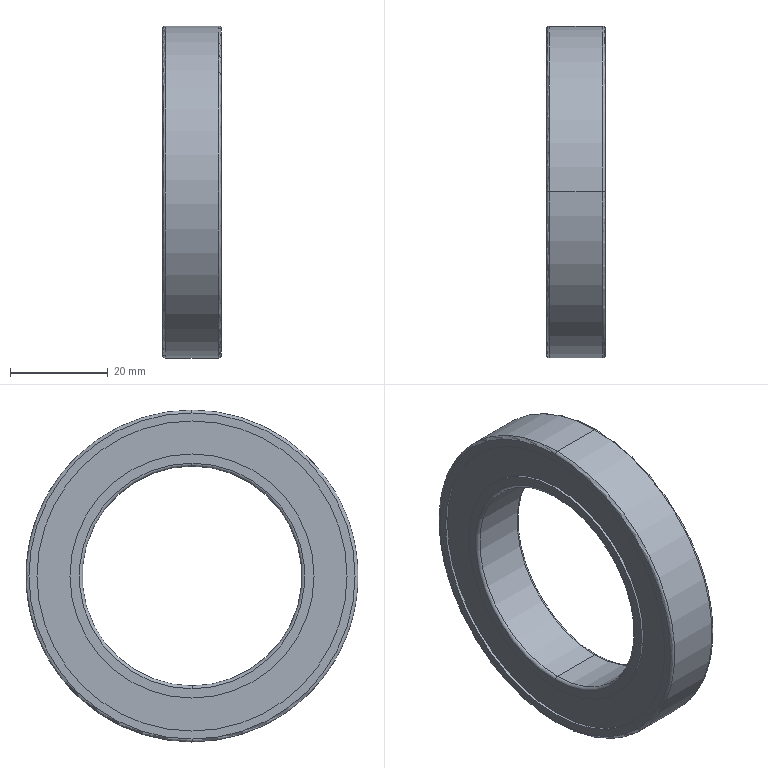Part | SolidWorks | features Fillet 2, Revolution 1 | 1 solid | 26 faces | box 12 x 68 x 68 mm | volume 23116 mm3 | cylinder 12 | torus 8 | plane 6 | commonest cylinder face diameters 50 x4 63.5 x4 45 x2 68 x2
STEP:
#1=CARTESIAN_POINT('',(0.6,0.,22.5));
#2=VERTEX_POINT('',#1);
#3=CARTESIAN_POINT('',(0.6,0.,-22.5));
#4=VERTEX_POINT('',#3);
#5=CARTESIAN_POINT('',(0.6,0.,0.));
#6=DIRECTION('',(-1.,0.,0.));
#7=DIRECTION('',(0.,0.,-1.));
#8=AXIS2_PLACEMENT_3D('',#5,#6,#7);
#9=CIRCLE('',#8,22.5);
#10=EDGE_CURVE('',#2,#4,#9,.T.);
#11=ORIENTED_EDGE('',*,*,#10,.F.);
#12=CARTESIAN_POINT('',(0.,0.,23.1));
#13=VERTEX_POINT('',#12);
#14=CARTESIAN_POINT('',(0.6,0.,23.1));
#15=DIRECTION('',(0.,1.,0.));
#16=DIRECTION('',(0.,0.,1.));
#17=AXIS2_PLACEMENT_3D('',#14,#15,#16);
#18=CIRCLE('',#17,0.6);
#19=EDGE_CURVE('',#2,#13,#18,.T.);
#20=ORIENTED_EDGE('',*,*,#19,.T.);
#21=CARTESIAN_POINT('',(0.,0.,-23.1));
#22=VERTEX_POINT('',#21);
#23=CARTESIAN_POINT('',(0.,0.,0.));
#24=DIRECTION('',(1.,0.,0.));
#25=DIRECTION('',(0.,0.,-1.));
#26=AXIS2_PLACEMENT_3D('',#23,#24,#25);
#27=CIRCLE('',#26,23.1);
#28=EDGE_CURVE('',#22,#13,#27,.T.);
#29=ORIENTED_EDGE('',*,*,#28,.F.);
#30=CARTESIAN_POINT('',(0.6,0.,-23.1));
#31=DIRECTION('',(0.,-1.,0.));
#32=DIRECTION('',(0.,0.,-1.));
#33=AXIS2_PLACEMENT_3D('',#30,#31,#32);
#34=CIRCLE('',#33,0.6);
#35=EDGE_CURVE('',#4,#22,#34,.T.);
#36=ORIENTED_EDGE('',*,*,#35,.F.);
#37=EDGE_LOOP('',(#11,#20,#29,#36));
#38=FACE_OUTER_BOUND('',#37,.T.);
#39=CARTESIAN_POINT('',(0.6,0.,0.));
#40=DIRECTION('',(1.,0.,0.));
#41=DIRECTION('',(0.,0.,-1.));
#42=AXIS2_PLACEMENT_3D('',#39,#40,#41);
#43=TOROIDAL_SURFACE('',#42,23.1,0.6);
#44=ADVANCED_FACE('',(#38),#43,.T.);
#45=CARTESIAN_POINT('',(11.4,0.,-22.5));
#46=VERTEX_POINT('',#45);
#47=CARTESIAN_POINT('',(11.4,0.,22.5));
#48=VERTEX_POINT('',#47);
#49=CARTESIAN_POINT('',(11.4,0.,0.));
#50=DIRECTION('',(1.,0.,0.));
#51=DIRECTION('',(0.,0.,1.));
#52=AXIS2_PLACEMENT_3D('',#49,#50,#51);
#53=CIRCLE('',#52,22.5);
#54=EDGE_CURVE('',#46,#48,#53,.T.);
#55=ORIENTED_EDGE('',*,*,#54,.F.);
#56=CARTESIAN_POINT('',(12.,0.,-23.1));
#57=VERTEX_POINT('',#56);
#58=CARTESIAN_POINT('',(11.4,0.,-23.1));
#59=DIRECTION('',(0.,1.,0.));
#60=DIRECTION('',(0.,0.,1.));
#61=AXIS2_PLACEMENT_3D('',#58,#59,#60);
#62=CIRCLE('',#61,0.6);
#63=EDGE_CURVE('',#46,#57,#62,.T.);
#64=ORIENTED_EDGE('',*,*,#63,.T.);
#65=CARTESIAN_POINT('',(12.,0.,23.1));
#66=VERTEX_POINT('',#65);
#67=CARTESIAN_POINT('',(12.,0.,0.));
#68=DIRECTION('',(-1.,0.,0.));
#69=DIRECTION('',(0.,0.,1.));
#70=AXIS2_PLACEMENT_3D('',#67,#68,#69);
#71=CIRCLE('',#70,23.1);
#72=EDGE_CURVE('',#66,#57,#71,.T.);
#73=ORIENTED_EDGE('',*,*,#72,.F.);
#74=CARTESIAN_POINT('',(11.4,0.,23.1));
#75=DIRECTION('',(0.,-1.,0.));
#76=DIRECTION('',(0.,0.,-1.));
#77=AXIS2_PLACEMENT_3D('',#74,#75,#76);
#78=CIRCLE('',#77,0.6);
#79=EDGE_CURVE('',#48,#66,#78,.T.);
#80=ORIENTED_EDGE('',*,*,#79,.F.);
#81=EDGE_LOOP('',(#55,#64,#73,#80));
#82=FACE_OUTER_BOUND('',#81,.T.);
#83=CARTESIAN_POINT('',(11.4,0.,0.));
#84=DIRECTION('',(-1.,0.,0.));
#85=DIRECTION('',(0.,0.,1.));
#86=AXIS2_PLACEMENT_3D('',#83,#84,#85);
#87=TOROIDAL_SURFACE('',#86,23.1,0.6);
#88=ADVANCED_FACE('',(#82),#87,.T.);
#89=CARTESIAN_POINT('',(0.,0.,33.4));
#90=VERTEX_POINT('',#89);
#91=CARTESIAN_POINT('',(0.,0.,-33.4));
#92=VERTEX_POINT('',#91);
#93=CARTESIAN_POINT('',(0.,0.,0.));
#94=DIRECTION('',(-1.,0.,0.));
#95=DIRECTION('',(0.,0.,-1.));
#96=AXIS2_PLACEMENT_3D('',#93,#94,#95);
#97=CIRCLE('',#96,33.4);
#98=EDGE_CURVE('',#90,#92,#97,.T.);
#99=ORIENTED_EDGE('',*,*,#98,.F.);
#100=CARTESIAN_POINT('',(0.6,0.,34.));
#101=VERTEX_POINT('',#100);
#102=CARTESIAN_POINT('',(0.6,0.,33.4));
#103=DIRECTION('',(0.,1.,0.));
#104=DIRECTION('',(0.,0.,1.));
#105=AXIS2_PLACEMENT_3D('',#102,#103,#104);
#106=CIRCLE('',#105,0.6);
#107=EDGE_CURVE('',#90,#101,#106,.T.);
#108=ORIENTED_EDGE('',*,*,#107,.T.);
#109=CARTESIAN_POINT('',(0.6,0.,-34.));
#110=VERTEX_POINT('',#109);
#111=CARTESIAN_POINT('',(0.6,0.,0.));
#112=DIRECTION('',(1.,0.,0.));
#113=DIRECTION('',(0.,0.,-1.));
#114=AXIS2_PLACEMENT_3D('',#111,#112,#113);
#115=CIRCLE('',#114,34.);
#116=EDGE_CURVE('',#110,#101,#115,.T.);
#117=ORIENTED_EDGE('',*,*,#116,.F.);
#118=CARTESIAN_POINT('',(0.6,0.,-33.4));
#119=DIRECTION('',(0.,-1.,0.));
#120=DIRECTION('',(0.,0.,-1.));
#121=AXIS2_PLACEMENT_3D('',#118,#119,#120);
#122=CIRCLE('',#121,0.6);
#123=EDGE_CURVE('',#92,#110,#122,.T.);
#124=ORIENTED_EDGE('',*,*,#123,.F.);
#125=EDGE_LOOP('',(#99,#108,#117,#124));
#126=FACE_OUTER_BOUND('',#125,.T.);
#127=CARTESIAN_POINT('',(0.6,0.,0.));
#128=DIRECTION('',(1.,0.,0.));
#129=DIRECTION('',(0.,0.,-1.));
#130=AXIS2_PLACEMENT_3D('',#127,#128,#129);
#131=TOROIDAL_SURFACE('',#130,33.4,0.6);
#132=ADVANCED_FACE('',(#126),#131,.T.);
#133=CARTESIAN_POINT('',(12.,0.,-33.4));
#134=VERTEX_POINT('',#133);
#135=CARTESIAN_POINT('',(12.,0.,33.4));
#136=VERTEX_POINT('',#135);
#137=CARTESIAN_POINT('',(12.,0.,0.));
#138=DIRECTION('',(1.,0.,0.));
#139=DIRECTION('',(0.,0.,1.));
#140=AXIS2_PLACEMENT_3D('',#137,#138,#139);
#141=CIRCLE('',#140,33.4);
#142=EDGE_CURVE('',#134,#136,#141,.T.);
#143=ORIENTED_EDGE('',*,*,#142,.F.);
#144=CARTESIAN_POINT('',(11.4,0.,-34.));
#145=VERTEX_POINT('',#144);
#146=CARTESIAN_POINT('',(11.4,0.,-33.4));
#147=DIRECTION('',(0.,1.,0.));
#148=DIRECTION('',(0.,0.,1.));
#149=AXIS2_PLACEMENT_3D('',#146,#147,#148);
#150=CIRCLE('',#149,0.6);
#151=EDGE_CURVE('',#134,#145,#150,.T.);
#152=ORIENTED_EDGE('',*,*,#151,.T.);
#153=CARTESIAN_POINT('',(11.4,0.,34.));
#154=VERTEX_POINT('',#153);
#155=CARTESIAN_POINT('',(11.4,0.,0.));
#156=DIRECTION('',(-1.,0.,0.));
#157=DIRECTION('',(0.,0.,1.));
#158=AXIS2_PLACEMENT_3D('',#155,#156,#157);
#159=CIRCLE('',#158,34.);
#160=EDGE_CURVE('',#154,#145,#159,.T.);
#161=ORIENTED_EDGE('',*,*,#160,.F.);
#162=CARTESIAN_POINT('',(11.4,0.,33.4));
#163=DIRECTION('',(0.,-1.,0.));
#164=DIRECTION('',(0.,0.,-1.));
#165=AXIS2_PLACEMENT_3D('',#162,#163,#164);
#166=CIRCLE('',#165,0.6);
#167=EDGE_CURVE('',#136,#154,#166,.T.);
#168=ORIENTED_EDGE('',*,*,#167,.F.);
#169=EDGE_LOOP('',(#143,#152,#161,#168));
#170=FACE_OUTER_BOUND('',#169,.T.);
#171=CARTESIAN_POINT('',(11.4,0.,0.));
#172=DIRECTION('',(-1.,0.,0.));
#173=DIRECTION('',(0.,0.,1.));
#174=AXIS2_PLACEMENT_3D('',#171,#172,#173);
#175=TOROIDAL_SURFACE('',#174,33.4,0.6);
#176=ADVANCED_FACE('',(#170),#175,.T.);
#177=ORIENTED_EDGE('',*,*,#160,.T.);
#178=CARTESIAN_POINT('',(0.,0.,-34.));
#179=DIRECTION('',(-1.,0.,0.));
#180=VECTOR('',#179,1000.);
#181=LINE('',#178,#180);
#182=EDGE_CURVE('',#145,#110,#181,.T.);
#183=ORIENTED_EDGE('',*,*,#182,.T.);
#184=ORIENTED_EDGE('',*,*,#116,.T.);
#185=CARTESIAN_POINT('',(0.,0.,34.));
#186=DIRECTION('',(-1.,0.,0.));
#187=VECTOR('',#186,1000.);
#188=LINE('',#185,#187);
#189=EDGE_CURVE('',#154,#101,#188,.T.);
#190=ORIENTED_EDGE('',*,*,#189,.F.);
#191=EDGE_LOOP('',(#177,#183,#184,#190));
#192=FACE_OUTER_BOUND('',#191,.T.);
#193=CARTESIAN_POINT('',(0.,0.,0.));
#194=DIRECTION('',(-1.,0.,0.));
#195=DIRECTION('',(0.,0.,1.));
#196=AXIS2_PLACEMENT_3D('',#193,#194,#195);
#197=CYLINDRICAL_SURFACE('',#196,34.);
#198=ADVANCED_FACE('',(#192),#197,.T.);
#199=CARTESIAN_POINT('',(12.,0.,-31.75));
#200=VERTEX_POINT('',#199);
#201=CARTESIAN_POINT('',(12.,0.,31.75));
#202=VERTEX_POINT('',#201);
#203=CARTESIAN_POINT('',(12.,0.,0.));
#204=DIRECTION('',(-1.,0.,0.));
#205=DIRECTION('',(0.,0.,1.));
#206=AXIS2_PLACEMENT_3D('',#203,#204,#205);
#207=CIRCLE('',#206,31.75);
#208=EDGE_CURVE('',#200,#202,#207,.T.);
#209=ORIENTED_EDGE('',*,*,#208,.F.);
#210=CARTESIAN_POINT('',(11.45,0.,-31.75));
#211=VERTEX_POINT('',#210);
#212=CARTESIAN_POINT('',(0.,0.,-31.75));
#213=DIRECTION('',(-1.,0.,0.));
#214=VECTOR('',#213,1000.);
#215=LINE('',#212,#214);
#216=EDGE_CURVE('',#200,#211,#215,.T.);
#217=ORIENTED_EDGE('',*,*,#216,.T.);
#218=CARTESIAN_POINT('',(11.45,0.,31.75));
#219=VERTEX_POINT('',#218);
#220=CARTESIAN_POINT('',(11.45,0.,0.));
#221=DIRECTION('',(-1.,0.,0.));
#222=DIRECTION('',(0.,0.,1.));
#223=AXIS2_PLACEMENT_3D('',#220,#221,#222);
#224=CIRCLE('',#223,31.75);
#225=EDGE_CURVE('',#211,#219,#224,.T.);
#226=ORIENTED_EDGE('',*,*,#225,.T.);
#227=CARTESIAN_POINT('',(0.,0.,31.75));
#228=DIRECTION('',(-1.,0.,0.));
#229=VECTOR('',#228,1000.);
#230=LINE('',#227,#229);
#231=EDGE_CURVE('',#202,#219,#230,.T.);
#232=ORIENTED_EDGE('',*,*,#231,.F.);
#233=EDGE_LOOP('',(#209,#217,#226,#232));
#234=FACE_OUTER_BOUND('',#233,.T.);
#235=CARTESIAN_POINT('',(0.,0.,0.));
#236=DIRECTION('',(-1.,0.,0.));
#237=DIRECTION('',(0.,0.,1.));
#238=AXIS2_PLACEMENT_3D('',#235,#236,#237);
#239=CYLINDRICAL_SURFACE('',#238,31.75);
#240=ADVANCED_FACE('',(#234),#239,.F.);
#241=CARTESIAN_POINT('',(12.,0.,25.));
#242=VERTEX_POINT('',#241);
#243=CARTESIAN_POINT('',(12.,0.,-25.));
#244=VERTEX_POINT('',#243);
#245=CARTESIAN_POINT('',(12.,0.,0.));
#246=DIRECTION('',(-1.,0.,0.));
#247=DIRECTION('',(0.,0.,1.));
#248=AXIS2_PLACEMENT_3D('',#245,#246,#247);
#249=CIRCLE('',#248,25.);
#250=EDGE_CURVE('',#242,#244,#249,.T.);
#251=ORIENTED_EDGE('',*,*,#250,.T.);
#252=CARTESIAN_POINT('',(11.45,0.,-25.));
#253=VERTEX_POINT('',#252);
#254=CARTESIAN_POINT('',(0.,0.,-25.));
#255=DIRECTION('',(-1.,0.,0.));
#256=VECTOR('',#255,1000.);
#257=LINE('',#254,#256);
#258=EDGE_CURVE('',#244,#253,#257,.T.);
#259=ORIENTED_EDGE('',*,*,#258,.T.);
#260=CARTESIAN_POINT('',(11.45,0.,25.));
#261=VERTEX_POINT('',#260);
#262=CARTESIAN_POINT('',(11.45,0.,0.));
#263=DIRECTION('',(-1.,0.,0.));
#264=DIRECTION('',(0.,0.,1.));
#265=AXIS2_PLACEMENT_3D('',#262,#263,#264);
#266=CIRCLE('',#265,25.);
#267=EDGE_CURVE('',#261,#253,#266,.T.);
#268=ORIENTED_EDGE('',*,*,#267,.F.);
#269=CARTESIAN_POINT('',(0.,0.,25.));
#270=DIRECTION('',(-1.,0.,0.));
#271=VECTOR('',#270,1000.);
#272=LINE('',#269,#271);
#273=EDGE_CURVE('',#242,#261,#272,.T.);
#274=ORIENTED_EDGE('',*,*,#273,.F.);
#275=EDGE_LOOP('',(#251,#259,#268,#274));
#276=FACE_OUTER_BOUND('',#275,.T.);
#277=CARTESIAN_POINT('',(0.,0.,0.));
#278=DIRECTION('',(-1.,0.,0.));
#279=DIRECTION('',(0.,0.,1.));
#280=AXIS2_PLACEMENT_3D('',#277,#278,#279);
#281=CYLINDRICAL_SURFACE('',#280,25.);
#282=ADVANCED_FACE('',(#276),#281,.T.);
#283=CARTESIAN_POINT('',(11.4,0.,0.));
#284=DIRECTION('',(1.,0.,0.));
#285=DIRECTION('',(0.,0.,1.));
#286=AXIS2_PLACEMENT_3D('',#283,#284,#285);
#287=CIRCLE('',#286,22.5);
#288=EDGE_CURVE('',#48,#46,#287,.T.);
#289=ORIENTED_EDGE('',*,*,#288,.T.);
#290=CARTESIAN_POINT('',(0.,0.,-22.5));
#291=DIRECTION('',(-1.,0.,0.));
#292=VECTOR('',#291,1000.);
#293=LINE('',#290,#292);
#294=EDGE_CURVE('',#46,#4,#293,.T.);
#295=ORIENTED_EDGE('',*,*,#294,.T.);
#296=CARTESIAN_POINT('',(0.6,0.,0.));
#297=DIRECTION('',(-1.,0.,0.));
#298=DIRECTION('',(0.,0.,-1.));
#299=AXIS2_PLACEMENT_3D('',#296,#297,#298);
#300=CIRCLE('',#299,22.5);
#301=EDGE_CURVE('',#4,#2,#300,.T.);
#302=ORIENTED_EDGE('',*,*,#301,.T.);
#303=CARTESIAN_POINT('',(0.,0.,22.5));
#304=DIRECTION('',(-1.,0.,0.));
#305=VECTOR('',#304,1000.);
#306=LINE('',#303,#305);
#307=EDGE_CURVE('',#48,#2,#306,.T.);
#308=ORIENTED_EDGE('',*,*,#307,.F.);
#309=EDGE_LOOP('',(#289,#295,#302,#308));
#310=FACE_OUTER_BOUND('',#309,.T.);
#311=CARTESIAN_POINT('',(0.,0.,0.));
#312=DIRECTION('',(-1.,0.,0.));
#313=DIRECTION('',(0.,0.,1.));
#314=AXIS2_PLACEMENT_3D('',#311,#312,#313);
#315=CYLINDRICAL_SURFACE('',#314,22.5);
#316=ADVANCED_FACE('',(#310),#315,.F.);
#317=CARTESIAN_POINT('',(0.55,0.,25.));
#318=VERTEX_POINT('',#317);
#319=CARTESIAN_POINT('',(0.55,0.,-25.));
#320=VERTEX_POINT('',#319);
#321=CARTESIAN_POINT('',(0.55,0.,0.));
#322=DIRECTION('',(-1.,0.,0.));
#323=DIRECTION('',(0.,0.,1.));
#324=AXIS2_PLACEMENT_3D('',#321,#322,#323);
#325=CIRCLE('',#324,25.);
#326=EDGE_CURVE('',#318,#320,#325,.T.);
#327=ORIENTED_EDGE('',*,*,#326,.T.);
#328=CARTESIAN_POINT('',(0.,0.,-25.));
#329=VERTEX_POINT('',#328);
#330=CARTESIAN_POINT('',(0.,0.,-25.));
#331=DIRECTION('',(-1.,0.,0.));
#332=VECTOR('',#331,1000.);
#333=LINE('',#330,#332);
#334=EDGE_CURVE('',#320,#329,#333,.T.);
#335=ORIENTED_EDGE('',*,*,#334,.T.);
#336=CARTESIAN_POINT('',(0.,0.,25.));
#337=VERTEX_POINT('',#336);
#338=CARTESIAN_POINT('',(0.,0.,0.));
#339=DIRECTION('',(-1.,0.,0.));
#340=DIRECTION('',(0.,0.,1.));
#341=AXIS2_PLACEMENT_3D('',#338,#339,#340);
#342=CIRCLE('',#341,25.);
#343=EDGE_CURVE('',#337,#329,#342,.T.);
#344=ORIENTED_EDGE('',*,*,#343,.F.);
#345=CARTESIAN_POINT('',(0.,0.,25.));
#346=DIRECTION('',(-1.,0.,0.));
#347=VECTOR('',#346,1000.);
#348=LINE('',#345,#347);
#349=EDGE_CURVE('',#318,#337,#348,.T.);
#350=ORIENTED_EDGE('',*,*,#349,.F.);
#351=EDGE_LOOP('',(#327,#335,#344,#350));
#352=FACE_OUTER_BOUND('',#351,.T.);
#353=CARTESIAN_POINT('',(0.,0.,0.));
#354=DIRECTION('',(-1.,0.,0.));
#355=DIRECTION('',(0.,0.,1.));
#356=AXIS2_PLACEMENT_3D('',#353,#354,#355);
#357=CYLINDRICAL_SURFACE('',#356,25.);
#358=ADVANCED_FACE('',(#352),#357,.T.);
#359=CARTESIAN_POINT('',(0.55,0.,-31.75));
#360=VERTEX_POINT('',#359);
#361=CARTESIAN_POINT('',(0.55,0.,31.75));
#362=VERTEX_POINT('',#361);
#363=CARTESIAN_POINT('',(0.55,0.,0.));
#364=DIRECTION('',(-1.,0.,0.));
#365=DIRECTION('',(0.,0.,1.));
#366=AXIS2_PLACEMENT_3D('',#363,#364,#365);
#367=CIRCLE('',#366,31.75);
#368=EDGE_CURVE('',#360,#362,#367,.T.);
#369=ORIENTED_EDGE('',*,*,#368,.F.);
#370=CARTESIAN_POINT('',(0.,0.,-31.75));
#371=VERTEX_POINT('',#370);
#372=CARTESIAN_POINT('',(0.,0.,-31.75));
#373=DIRECTION('',(-1.,0.,0.));
#374=VECTOR('',#373,1000.);
#375=LINE('',#372,#374);
#376=EDGE_CURVE('',#360,#371,#375,.T.);
#377=ORIENTED_EDGE('',*,*,#376,.T.);
#378=CARTESIAN_POINT('',(0.,0.,31.75));
#379=VERTEX_POINT('',#378);
#380=CARTESIAN_POINT('',(0.,0.,0.));
#381=DIRECTION('',(-1.,0.,0.));
#382=DIRECTION('',(0.,0.,1.));
#383=AXIS2_PLACEMENT_3D('',#380,#381,#382);
#384=CIRCLE('',#383,31.75);
#385=EDGE_CURVE('',#371,#379,#384,.T.);
#386=ORIENTED_EDGE('',*,*,#385,.T.);
#387=CARTESIAN_POINT('',(0.,0.,31.75));
#388=DIRECTION('',(-1.,0.,0.));
#389=VECTOR('',#388,1000.);
#390=LINE('',#387,#389);
#391=EDGE_CURVE('',#362,#379,#390,.T.);
#392=ORIENTED_EDGE('',*,*,#391,.F.);
#393=EDGE_LOOP('',(#369,#377,#386,#392));
#394=FACE_OUTER_BOUND('',#393,.T.);
#395=CARTESIAN_POINT('',(0.,0.,0.));
#396=DIRECTION('',(-1.,0.,0.));
#397=DIRECTION('',(0.,0.,1.));
#398=AXIS2_PLACEMENT_3D('',#395,#396,#397);
#399=CYLINDRICAL_SURFACE('',#398,31.75);
#400=ADVANCED_FACE('',(#394),#399,.F.);
#401=CARTESIAN_POINT('',(0.,0.,0.));
#402=DIRECTION('',(-1.,0.,0.));
#403=DIRECTION('',(0.,0.,-1.));
#404=AXIS2_PLACEMENT_3D('',#401,#402,#403);
#405=CIRCLE('',#404,33.4);
#406=EDGE_CURVE('',#92,#90,#405,.T.);
#407=ORIENTED_EDGE('',*,*,#406,.T.);
#408=ORIENTED_EDGE('',*,*,#98,.T.);
#409=EDGE_LOOP('',(#407,#408));
#410=FACE_OUTER_BOUND('',#409,.T.);
#411=CARTESIAN_POINT('',(0.,0.,0.));
#412=DIRECTION('',(-1.,0.,0.));
#413=DIRECTION('',(0.,0.,1.));
#414=AXIS2_PLACEMENT_3D('',#411,#412,#413);
#415=CIRCLE('',#414,31.75);
#416=EDGE_CURVE('',#379,#371,#415,.T.);
#417=ORIENTED_EDGE('',*,*,#416,.F.);
#418=ORIENTED_EDGE('',*,*,#385,.F.);
#419=EDGE_LOOP('',(#417,#418));
#420=FACE_BOUND('',#419,.T.);
#421=CARTESIAN_POINT('',(0.,34.,0.));
#422=DIRECTION('',(1.,0.,0.));
#423=DIRECTION('',(0.,0.,-1.));
#424=AXIS2_PLACEMENT_3D('',#421,#422,#423);
#425=PLANE('',#424);
#426=ADVANCED_FACE('',(#410,#420),#425,.F.);
#427=ORIENTED_EDGE('',*,*,#376,.F.);
#428=CARTESIAN_POINT('',(0.55,0.,0.));
#429=DIRECTION('',(-1.,0.,0.));
#430=DIRECTION('',(0.,0.,1.));
#431=AXIS2_PLACEMENT_3D('',#428,#429,#430);
#432=CIRCLE('',#431,31.75);
#433=EDGE_CURVE('',#362,#360,#432,.T.);
#434=ORIENTED_EDGE('',*,*,#433,.F.);
#435=ORIENTED_EDGE('',*,*,#391,.T.);
#436=ORIENTED_EDGE('',*,*,#416,.T.);
#437=EDGE_LOOP('',(#427,#434,#435,#436));
#438=FACE_OUTER_BOUND('',#437,.T.);
#439=CARTESIAN_POINT('',(0.,0.,0.));
#440=DIRECTION('',(-1.,0.,0.));
#441=DIRECTION('',(0.,0.,1.));
#442=AXIS2_PLACEMENT_3D('',#439,#440,#441);
#443=CYLINDRICAL_SURFACE('',#442,31.75);
#444=ADVANCED_FACE('',(#438),#443,.F.);
#445=ORIENTED_EDGE('',*,*,#326,.F.);
#446=CARTESIAN_POINT('',(0.55,0.,0.));
#447=DIRECTION('',(-1.,0.,0.));
#448=DIRECTION('',(0.,0.,1.));
#449=AXIS2_PLACEMENT_3D('',#446,#447,#448);
#450=CIRCLE('',#449,25.);
#451=EDGE_CURVE('',#320,#318,#450,.T.);
#452=ORIENTED_EDGE('',*,*,#451,.F.);
#453=EDGE_LOOP('',(#445,#452));
#454=FACE_BOUND('',#453,.T.);
#455=ORIENTED_EDGE('',*,*,#433,.T.);
#456=ORIENTED_EDGE('',*,*,#368,.T.);
#457=EDGE_LOOP('',(#455,#456));
#458=FACE_OUTER_BOUND('',#457,.T.);
#459=CARTESIAN_POINT('',(0.55,31.75,0.));
#460=DIRECTION('',(1.,0.,0.));
#461=DIRECTION('',(0.,0.,-1.));
#462=AXIS2_PLACEMENT_3D('',#459,#460,#461);
#463=PLANE('',#462);
#464=ADVANCED_FACE('',(#454,#458),#463,.F.);
#465=ORIENTED_EDGE('',*,*,#334,.F.);
#466=ORIENTED_EDGE('',*,*,#451,.T.);
#467=ORIENTED_EDGE('',*,*,#349,.T.);
#468=CARTESIAN_POINT('',(0.,0.,0.));
#469=DIRECTION('',(-1.,0.,0.));
#470=DIRECTION('',(0.,0.,1.));
#471=AXIS2_PLACEMENT_3D('',#468,#469,#470);
#472=CIRCLE('',#471,25.);
#473=EDGE_CURVE('',#329,#337,#472,.T.);
#474=ORIENTED_EDGE('',*,*,#473,.F.);
#475=EDGE_LOOP('',(#465,#466,#467,#474));
#476=FACE_OUTER_BOUND('',#475,.T.);
#477=CARTESIAN_POINT('',(0.,0.,0.));
#478=DIRECTION('',(-1.,0.,0.));
#479=DIRECTION('',(0.,0.,1.));
#480=AXIS2_PLACEMENT_3D('',#477,#478,#479);
#481=CYLINDRICAL_SURFACE('',#480,25.);
#482=ADVANCED_FACE('',(#476),#481,.T.);
#483=ORIENTED_EDGE('',*,*,#28,.T.);
#484=CARTESIAN_POINT('',(0.,0.,0.));
#485=DIRECTION('',(1.,0.,0.));
#486=DIRECTION('',(0.,0.,-1.));
#487=AXIS2_PLACEMENT_3D('',#484,#485,#486);
#488=CIRCLE('',#487,23.1);
#489=EDGE_CURVE('',#13,#22,#488,.T.);
#490=ORIENTED_EDGE('',*,*,#489,.T.);
#491=EDGE_LOOP('',(#483,#490));
#492=FACE_BOUND('',#491,.T.);
#493=ORIENTED_EDGE('',*,*,#343,.T.);
#494=ORIENTED_EDGE('',*,*,#473,.T.);
#495=EDGE_LOOP('',(#493,#494));
#496=FACE_OUTER_BOUND('',#495,.T.);
#497=CARTESIAN_POINT('',(0.,25.,0.));
#498=DIRECTION('',(1.,0.,0.));
#499=DIRECTION('',(0.,0.,-1.));
#500=AXIS2_PLACEMENT_3D('',#497,#498,#499);
#501=PLANE('',#500);
#502=ADVANCED_FACE('',(#492,#496),#501,.F.);
#503=ORIENTED_EDGE('',*,*,#294,.F.);
#504=ORIENTED_EDGE('',*,*,#54,.T.);
#505=ORIENTED_EDGE('',*,*,#307,.T.);
#506=ORIENTED_EDGE('',*,*,#10,.T.);
#507=EDGE_LOOP('',(#503,#504,#505,#506));
#508=FACE_OUTER_BOUND('',#507,.T.);
#509=CARTESIAN_POINT('',(0.,0.,0.));
#510=DIRECTION('',(-1.,0.,0.));
#511=DIRECTION('',(0.,0.,1.));
#512=AXIS2_PLACEMENT_3D('',#509,#510,#511);
#513=CYLINDRICAL_SURFACE('',#512,22.5);
#514=ADVANCED_FACE('',(#508),#513,.F.);
#515=ORIENTED_EDGE('',*,*,#72,.T.);
#516=CARTESIAN_POINT('',(12.,0.,0.));
#517=DIRECTION('',(-1.,0.,0.));
#518=DIRECTION('',(0.,0.,1.));
#519=AXIS2_PLACEMENT_3D('',#516,#517,#518);
#520=CIRCLE('',#519,23.1);
#521=EDGE_CURVE('',#57,#66,#520,.T.);
#522=ORIENTED_EDGE('',*,*,#521,.T.);
#523=EDGE_LOOP('',(#515,#522));
#524=FACE_BOUND('',#523,.T.);
#525=ORIENTED_EDGE('',*,*,#250,.F.);
#526=CARTESIAN_POINT('',(12.,0.,0.));
#527=DIRECTION('',(-1.,0.,0.));
#528=DIRECTION('',(0.,0.,1.));
#529=AXIS2_PLACEMENT_3D('',#526,#527,#528);
#530=CIRCLE('',#529,25.);
#531=EDGE_CURVE('',#244,#242,#530,.T.);
#532=ORIENTED_EDGE('',*,*,#531,.F.);
#533=EDGE_LOOP('',(#525,#532));
#534=FACE_OUTER_BOUND('',#533,.T.);
#535=CARTESIAN_POINT('',(12.,25.,0.));
#536=DIRECTION('',(-1.,0.,0.));
#537=DIRECTION('',(0.,0.,1.));
#538=AXIS2_PLACEMENT_3D('',#535,#536,#537);
#539=PLANE('',#538);
#540=ADVANCED_FACE('',(#524,#534),#539,.F.);
#541=ORIENTED_EDGE('',*,*,#258,.F.);
#542=ORIENTED_EDGE('',*,*,#531,.T.);
#543=ORIENTED_EDGE('',*,*,#273,.T.);
#544=CARTESIAN_POINT('',(11.45,0.,0.));
#545=DIRECTION('',(-1.,0.,0.));
#546=DIRECTION('',(0.,0.,1.));
#547=AXIS2_PLACEMENT_3D('',#544,#545,#546);
#548=CIRCLE('',#547,25.);
#549=EDGE_CURVE('',#253,#261,#548,.T.);
#550=ORIENTED_EDGE('',*,*,#549,.F.);
#551=EDGE_LOOP('',(#541,#542,#543,#550));
#552=FACE_OUTER_BOUND('',#551,.T.);
#553=CARTESIAN_POINT('',(0.,0.,0.));
#554=DIRECTION('',(-1.,0.,0.));
#555=DIRECTION('',(0.,0.,1.));
#556=AXIS2_PLACEMENT_3D('',#553,#554,#555);
#557=CYLINDRICAL_SURFACE('',#556,25.);
#558=ADVANCED_FACE('',(#552),#557,.T.);
#559=CARTESIAN_POINT('',(11.45,0.,0.));
#560=DIRECTION('',(-1.,0.,0.));
#561=DIRECTION('',(0.,0.,1.));
#562=AXIS2_PLACEMENT_3D('',#559,#560,#561);
#563=CIRCLE('',#562,31.75);
#564=EDGE_CURVE('',#219,#211,#563,.T.);
#565=ORIENTED_EDGE('',*,*,#564,.F.);
#566=ORIENTED_EDGE('',*,*,#225,.F.);
#567=EDGE_LOOP('',(#565,#566));
#568=FACE_OUTER_BOUND('',#567,.T.);
#569=ORIENTED_EDGE('',*,*,#267,.T.);
#570=ORIENTED_EDGE('',*,*,#549,.T.);
#571=EDGE_LOOP('',(#569,#570));
#572=FACE_BOUND('',#571,.T.);
#573=CARTESIAN_POINT('',(11.45,31.75,0.));
#574=DIRECTION('',(-1.,0.,0.));
#575=DIRECTION('',(0.,0.,1.));
#576=AXIS2_PLACEMENT_3D('',#573,#574,#575);
#577=PLANE('',#576);
#578=ADVANCED_FACE('',(#568,#572),#577,.F.);
#579=ORIENTED_EDGE('',*,*,#216,.F.);
#580=CARTESIAN_POINT('',(12.,0.,0.));
#581=DIRECTION('',(-1.,0.,0.));
#582=DIRECTION('',(0.,0.,1.));
#583=AXIS2_PLACEMENT_3D('',#580,#581,#582);
#584=CIRCLE('',#583,31.75);
#585=EDGE_CURVE('',#202,#200,#584,.T.);
#586=ORIENTED_EDGE('',*,*,#585,.F.);
#587=ORIENTED_EDGE('',*,*,#231,.T.);
#588=ORIENTED_EDGE('',*,*,#564,.T.);
#589=EDGE_LOOP('',(#579,#586,#587,#588));
#590=FACE_OUTER_BOUND('',#589,.T.);
#591=CARTESIAN_POINT('',(0.,0.,0.));
#592=DIRECTION('',(-1.,0.,0.));
#593=DIRECTION('',(0.,0.,1.));
#594=AXIS2_PLACEMENT_3D('',#591,#592,#593);
#595=CYLINDRICAL_SURFACE('',#594,31.75);
#596=ADVANCED_FACE('',(#590),#595,.F.);
#597=CARTESIAN_POINT('',(12.,0.,0.));
#598=DIRECTION('',(1.,0.,0.));
#599=DIRECTION('',(0.,0.,1.));
#600=AXIS2_PLACEMENT_3D('',#597,#598,#599);
#601=CIRCLE('',#600,33.4);
#602=EDGE_CURVE('',#136,#134,#601,.T.);
#603=ORIENTED_EDGE('',*,*,#602,.T.);
#604=ORIENTED_EDGE('',*,*,#142,.T.);
#605=EDGE_LOOP('',(#603,#604));
#606=FACE_OUTER_BOUND('',#605,.T.);
#607=ORIENTED_EDGE('',*,*,#585,.T.);
#608=ORIENTED_EDGE('',*,*,#208,.T.);
#609=EDGE_LOOP('',(#607,#608));
#610=FACE_BOUND('',#609,.T.);
#611=CARTESIAN_POINT('',(12.,34.,0.));
#612=DIRECTION('',(-1.,0.,0.));
#613=DIRECTION('',(0.,0.,1.));
#614=AXIS2_PLACEMENT_3D('',#611,#612,#613);
#615=PLANE('',#614);
#616=ADVANCED_FACE('',(#606,#610),#615,.F.);
#617=ORIENTED_EDGE('',*,*,#182,.F.);
#618=CARTESIAN_POINT('',(11.4,0.,0.));
#619=DIRECTION('',(-1.,0.,0.));
#620=DIRECTION('',(0.,0.,1.));
#621=AXIS2_PLACEMENT_3D('',#618,#619,#620);
#622=CIRCLE('',#621,34.);
#623=EDGE_CURVE('',#145,#154,#622,.T.);
#624=ORIENTED_EDGE('',*,*,#623,.T.);
#625=ORIENTED_EDGE('',*,*,#189,.T.);
#626=CARTESIAN_POINT('',(0.6,0.,0.));
#627=DIRECTION('',(1.,0.,0.));
#628=DIRECTION('',(0.,0.,-1.));
#629=AXIS2_PLACEMENT_3D('',#626,#627,#628);
#630=CIRCLE('',#629,34.);
#631=EDGE_CURVE('',#101,#110,#630,.T.);
#632=ORIENTED_EDGE('',*,*,#631,.T.);
#633=EDGE_LOOP('',(#617,#624,#625,#632));
#634=FACE_OUTER_BOUND('',#633,.T.);
#635=CARTESIAN_POINT('',(0.,0.,0.));
#636=DIRECTION('',(-1.,0.,0.));
#637=DIRECTION('',(0.,0.,1.));
#638=AXIS2_PLACEMENT_3D('',#635,#636,#637);
#639=CYLINDRICAL_SURFACE('',#638,34.);
#640=ADVANCED_FACE('',(#634),#639,.T.);
#641=ORIENTED_EDGE('',*,*,#151,.F.);
#642=ORIENTED_EDGE('',*,*,#602,.F.);
#643=ORIENTED_EDGE('',*,*,#167,.T.);
#644=ORIENTED_EDGE('',*,*,#623,.F.);
#645=EDGE_LOOP('',(#641,#642,#643,#644));
#646=FACE_OUTER_BOUND('',#645,.T.);
#647=CARTESIAN_POINT('',(11.4,0.,0.));
#648=DIRECTION('',(-1.,0.,0.));
#649=DIRECTION('',(0.,0.,1.));
#650=AXIS2_PLACEMENT_3D('',#647,#648,#649);
#651=TOROIDAL_SURFACE('',#650,33.4,0.6);
#652=ADVANCED_FACE('',(#646),#651,.T.);
#653=ORIENTED_EDGE('',*,*,#107,.F.);
#654=ORIENTED_EDGE('',*,*,#406,.F.);
#655=ORIENTED_EDGE('',*,*,#123,.T.);
#656=ORIENTED_EDGE('',*,*,#631,.F.);
#657=EDGE_LOOP('',(#653,#654,#655,#656));
#658=FACE_OUTER_BOUND('',#657,.T.);
#659=CARTESIAN_POINT('',(0.6,0.,0.));
#660=DIRECTION('',(1.,0.,0.));
#661=DIRECTION('',(0.,0.,-1.));
#662=AXIS2_PLACEMENT_3D('',#659,#660,#661);
#663=TOROIDAL_SURFACE('',#662,33.4,0.6);
#664=ADVANCED_FACE('',(#658),#663,.T.);
#665=ORIENTED_EDGE('',*,*,#63,.F.);
#666=ORIENTED_EDGE('',*,*,#288,.F.);
#667=ORIENTED_EDGE('',*,*,#79,.T.);
#668=ORIENTED_EDGE('',*,*,#521,.F.);
#669=EDGE_LOOP('',(#665,#666,#667,#668));
#670=FACE_OUTER_BOUND('',#669,.T.);
#671=CARTESIAN_POINT('',(11.4,0.,0.));
#672=DIRECTION('',(-1.,0.,0.));
#673=DIRECTION('',(0.,0.,1.));
#674=AXIS2_PLACEMENT_3D('',#671,#672,#673);
#675=TOROIDAL_SURFACE('',#674,23.1,0.6);
#676=ADVANCED_FACE('',(#670),#675,.T.);
#677=ORIENTED_EDGE('',*,*,#19,.F.);
#678=ORIENTED_EDGE('',*,*,#301,.F.);
#679=ORIENTED_EDGE('',*,*,#35,.T.);
#680=ORIENTED_EDGE('',*,*,#489,.F.);
#681=EDGE_LOOP('',(#677,#678,#679,#680));
#682=FACE_OUTER_BOUND('',#681,.T.);
#683=CARTESIAN_POINT('',(0.6,0.,0.));
#684=DIRECTION('',(1.,0.,0.));
#685=DIRECTION('',(0.,0.,-1.));
#686=AXIS2_PLACEMENT_3D('',#683,#684,#685);
#687=TOROIDAL_SURFACE('',#686,23.1,0.6);
#688=ADVANCED_FACE('',(#682),#687,.T.);
#689=CLOSED_SHELL('',(#44,#88,#132,#176,#198,#240,#282,#316,#358,#400,#426,#444,#464,#482,#502,#514,#540,#558,#578,#596,#616,#640,#652,#664,#676,#688));
#690=MANIFOLD_SOLID_BREP('',#689);
#691=CARTESIAN_POINT('',(0.,0.,0.));
#692=DIRECTION('',(0.,0.,1.));
#693=DIRECTION('',(1.,0.,0.));
#694=AXIS2_PLACEMENT_3D('',#691,#692,#693);
#695=(LENGTH_UNIT()NAMED_UNIT(*)SI_UNIT(.MILLI.,.METRE.));
#696=UNCERTAINTY_MEASURE_WITH_UNIT(LENGTH_MEASURE(0.00001),#695,'','');
#697=(NAMED_UNIT(*)PLANE_ANGLE_UNIT()SI_UNIT($,.RADIAN.));
#698=(NAMED_UNIT(*)SI_UNIT($,.STERADIAN.)SOLID_ANGLE_UNIT());
#699=(GEOMETRIC_REPRESENTATION_CONTEXT(3)GLOBAL_UNCERTAINTY_ASSIGNED_CONTEXT((#696))GLOBAL_UNIT_ASSIGNED_CONTEXT((#695,#697,#698))REPRESENTATION_CONTEXT('',''));
#700=ADVANCED_BREP_SHAPE_REPRESENTATION('',(#690,#694),#699);